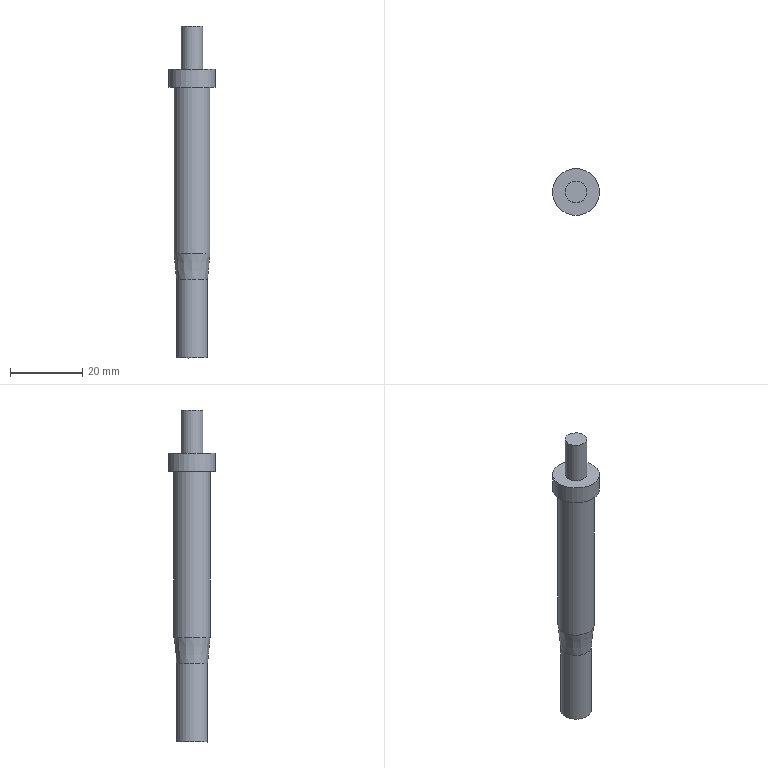Part | NX | features solid 2 | 1 solid | 9 faces | box 13 x 13 x 92 mm | volume 6374 mm3 | plane 4 | cylinder 4 | cone 1 | commonest cylinder face diameters 6 x1 8.6 x1 10 x1 13 x1
STEP:
#1=CARTESIAN_POINT('',(782.096,-115.667,54.));
#2=VERTEX_POINT('',#1);
#3=CARTESIAN_POINT('',(782.096,-119.967,54.));
#4=DIRECTION('',(0.,0.,1.));
#5=DIRECTION('',(0.,1.,0.));
#6=AXIS2_PLACEMENT_3D('',#3,#4,#5);
#7=CIRCLE('',#6,4.3);
#8=EDGE_CURVE('',#2,#2,#7,.F.);
#9=ORIENTED_EDGE('',*,*,#8,.T.);
#10=EDGE_LOOP('',(#9));
#11=FACE_BOUND('',#10,.T.);
#12=CARTESIAN_POINT('',(782.096,-119.967,54.));
#13=DIRECTION('',(0.,0.,-1.));
#14=DIRECTION('',(0.,1.,0.));
#15=AXIS2_PLACEMENT_3D('',#12,#13,#14);
#16=PLANE('',#15);
#17=ADVANCED_FACE('',(#11),#16,.T.);
#18=CARTESIAN_POINT('',(782.096,-124.267,75.632));
#19=VERTEX_POINT('',#18);
#20=CARTESIAN_POINT('',(782.096,-119.967,75.632));
#21=DIRECTION('',(0.,0.,-1.));
#22=DIRECTION('',(0.,-1.,0.));
#23=AXIS2_PLACEMENT_3D('',#20,#21,#22);
#24=CIRCLE('',#23,4.3);
#25=EDGE_CURVE('',#19,#19,#24,.T.);
#26=ORIENTED_EDGE('',*,*,#25,.T.);
#27=EDGE_LOOP('',(#26));
#28=FACE_BOUND('',#27,.T.);
#29=ORIENTED_EDGE('',*,*,#8,.F.);
#30=EDGE_LOOP('',(#29));
#31=FACE_BOUND('',#30,.T.);
#32=CARTESIAN_POINT('',(782.096,-119.967,54.));
#33=DIRECTION('',(0.,0.,1.));
#34=DIRECTION('',(0.,-1.,0.));
#35=AXIS2_PLACEMENT_3D('',#32,#33,#34);
#36=CYLINDRICAL_SURFACE('',#35,4.3);
#37=ADVANCED_FACE('',(#28,#31),#36,.T.);
#38=ORIENTED_EDGE('',*,*,#25,.F.);
#39=EDGE_LOOP('',(#38));
#40=FACE_BOUND('',#39,.T.);
#41=CARTESIAN_POINT('',(782.096,-124.967,83.));
#42=VERTEX_POINT('',#41);
#43=CARTESIAN_POINT('',(782.096,-119.967,83.));
#44=DIRECTION('',(0.,0.,-1.));
#45=DIRECTION('',(0.,-1.,0.));
#46=AXIS2_PLACEMENT_3D('',#43,#44,#45);
#47=CIRCLE('',#46,5.);
#48=EDGE_CURVE('',#42,#42,#47,.T.);
#49=ORIENTED_EDGE('',*,*,#48,.T.);
#50=EDGE_LOOP('',(#49));
#51=FACE_BOUND('',#50,.T.);
#52=CARTESIAN_POINT('',(782.096,-119.967,73.));
#53=DIRECTION('',(0.,0.,1.));
#54=DIRECTION('',(0.,-1.,0.));
#55=AXIS2_PLACEMENT_3D('',#52,#53,#54);
#56=CONICAL_SURFACE('',#55,4.05,0.09472);
#57=ADVANCED_FACE('',(#40,#51),#56,.T.);
#58=CARTESIAN_POINT('',(782.096,-114.967,129.));
#59=VERTEX_POINT('',#58);
#60=CARTESIAN_POINT('',(782.096,-119.967,129.));
#61=DIRECTION('',(0.,0.,1.));
#62=DIRECTION('',(0.,1.,0.));
#63=AXIS2_PLACEMENT_3D('',#60,#61,#62);
#64=CIRCLE('',#63,5.);
#65=EDGE_CURVE('',#59,#59,#64,.F.);
#66=ORIENTED_EDGE('',*,*,#65,.T.);
#67=EDGE_LOOP('',(#66));
#68=FACE_BOUND('',#67,.T.);
#69=ORIENTED_EDGE('',*,*,#48,.F.);
#70=EDGE_LOOP('',(#69));
#71=FACE_BOUND('',#70,.T.);
#72=CARTESIAN_POINT('',(782.096,-119.967,83.));
#73=DIRECTION('',(0.,0.,1.));
#74=DIRECTION('',(0.,-1.,0.));
#75=AXIS2_PLACEMENT_3D('',#72,#73,#74);
#76=CYLINDRICAL_SURFACE('',#75,5.);
#77=ADVANCED_FACE('',(#68,#71),#76,.T.);
#78=CARTESIAN_POINT('',(782.096,-122.967,134.));
#79=VERTEX_POINT('',#78);
#80=CARTESIAN_POINT('',(782.096,-119.967,134.));
#81=DIRECTION('',(0.,0.,-1.));
#82=DIRECTION('',(0.,-1.,0.));
#83=AXIS2_PLACEMENT_3D('',#80,#81,#82);
#84=CIRCLE('',#83,3.);
#85=EDGE_CURVE('',#79,#79,#84,.T.);
#86=ORIENTED_EDGE('',*,*,#85,.T.);
#87=EDGE_LOOP('',(#86));
#88=FACE_BOUND('',#87,.T.);
#89=CARTESIAN_POINT('',(782.096,-113.467,134.));
#90=VERTEX_POINT('',#89);
#91=CARTESIAN_POINT('',(782.096,-119.967,134.));
#92=DIRECTION('',(0.,0.,1.));
#93=DIRECTION('',(0.,1.,0.));
#94=AXIS2_PLACEMENT_3D('',#91,#92,#93);
#95=CIRCLE('',#94,6.5);
#96=EDGE_CURVE('',#90,#90,#95,.T.);
#97=ORIENTED_EDGE('',*,*,#96,.T.);
#98=EDGE_LOOP('',(#97));
#99=FACE_BOUND('',#98,.T.);
#100=CARTESIAN_POINT('',(782.096,-119.967,134.));
#101=DIRECTION('',(0.,0.,1.));
#102=DIRECTION('',(0.,-1.,0.));
#103=AXIS2_PLACEMENT_3D('',#100,#101,#102);
#104=PLANE('',#103);
#105=ADVANCED_FACE('',(#88,#99),#104,.T.);
#106=ORIENTED_EDGE('',*,*,#65,.F.);
#107=EDGE_LOOP('',(#106));
#108=FACE_BOUND('',#107,.T.);
#109=CARTESIAN_POINT('',(782.096,-126.467,129.));
#110=VERTEX_POINT('',#109);
#111=CARTESIAN_POINT('',(782.096,-119.967,129.));
#112=DIRECTION('',(0.,0.,-1.));
#113=DIRECTION('',(0.,-1.,0.));
#114=AXIS2_PLACEMENT_3D('',#111,#112,#113);
#115=CIRCLE('',#114,6.5);
#116=EDGE_CURVE('',#110,#110,#115,.T.);
#117=ORIENTED_EDGE('',*,*,#116,.T.);
#118=EDGE_LOOP('',(#117));
#119=FACE_BOUND('',#118,.T.);
#120=CARTESIAN_POINT('',(782.096,-119.967,129.));
#121=DIRECTION('',(0.,0.,-1.));
#122=DIRECTION('',(0.,1.,0.));
#123=AXIS2_PLACEMENT_3D('',#120,#121,#122);
#124=PLANE('',#123);
#125=ADVANCED_FACE('',(#108,#119),#124,.T.);
#126=ORIENTED_EDGE('',*,*,#96,.F.);
#127=EDGE_LOOP('',(#126));
#128=FACE_BOUND('',#127,.T.);
#129=ORIENTED_EDGE('',*,*,#116,.F.);
#130=EDGE_LOOP('',(#129));
#131=FACE_BOUND('',#130,.T.);
#132=CARTESIAN_POINT('',(782.096,-119.967,139.));
#133=DIRECTION('',(0.,0.,1.));
#134=DIRECTION('',(0.,-1.,0.));
#135=AXIS2_PLACEMENT_3D('',#132,#133,#134);
#136=CYLINDRICAL_SURFACE('',#135,6.5);
#137=ADVANCED_FACE('',(#128,#131),#136,.T.);
#138=CARTESIAN_POINT('',(782.096,-116.967,146.));
#139=VERTEX_POINT('',#138);
#140=CARTESIAN_POINT('',(782.096,-119.967,146.));
#141=DIRECTION('',(0.,0.,1.));
#142=DIRECTION('',(0.,1.,0.));
#143=AXIS2_PLACEMENT_3D('',#140,#141,#142);
#144=CIRCLE('',#143,3.);
#145=EDGE_CURVE('',#139,#139,#144,.T.);
#146=ORIENTED_EDGE('',*,*,#145,.T.);
#147=EDGE_LOOP('',(#146));
#148=FACE_BOUND('',#147,.T.);
#149=CARTESIAN_POINT('',(782.096,-119.967,146.));
#150=DIRECTION('',(0.,0.,1.));
#151=DIRECTION('',(0.,-1.,0.));
#152=AXIS2_PLACEMENT_3D('',#149,#150,#151);
#153=PLANE('',#152);
#154=ADVANCED_FACE('',(#148),#153,.T.);
#155=ORIENTED_EDGE('',*,*,#145,.F.);
#156=EDGE_LOOP('',(#155));
#157=FACE_BOUND('',#156,.T.);
#158=ORIENTED_EDGE('',*,*,#85,.F.);
#159=EDGE_LOOP('',(#158));
#160=FACE_BOUND('',#159,.T.);
#161=CARTESIAN_POINT('',(782.096,-119.967,144.));
#162=DIRECTION('',(0.,0.,1.));
#163=DIRECTION('',(0.,-1.,0.));
#164=AXIS2_PLACEMENT_3D('',#161,#162,#163);
#165=CYLINDRICAL_SURFACE('',#164,3.);
#166=ADVANCED_FACE('',(#157,#160),#165,.T.);
#167=CLOSED_SHELL('',(#17,#37,#57,#77,#105,#125,#137,#154,#166));
#168=MANIFOLD_SOLID_BREP('',#167);
#169=(LENGTH_UNIT()NAMED_UNIT(*)SI_UNIT(.MILLI.,.METRE.));
#170=UNCERTAINTY_MEASURE_WITH_UNIT(LENGTH_MEASURE(0.00001),#169,'','');
#171=(NAMED_UNIT(*)PLANE_ANGLE_UNIT()SI_UNIT($,.RADIAN.));
#172=(NAMED_UNIT(*)SI_UNIT($,.STERADIAN.)SOLID_ANGLE_UNIT());
#173=(GEOMETRIC_REPRESENTATION_CONTEXT(3)GLOBAL_UNCERTAINTY_ASSIGNED_CONTEXT((#170))GLOBAL_UNIT_ASSIGNED_CONTEXT((#169,#171,#172))REPRESENTATION_CONTEXT('',''));
#174=ADVANCED_BREP_SHAPE_REPRESENTATION('',(#168),#173);